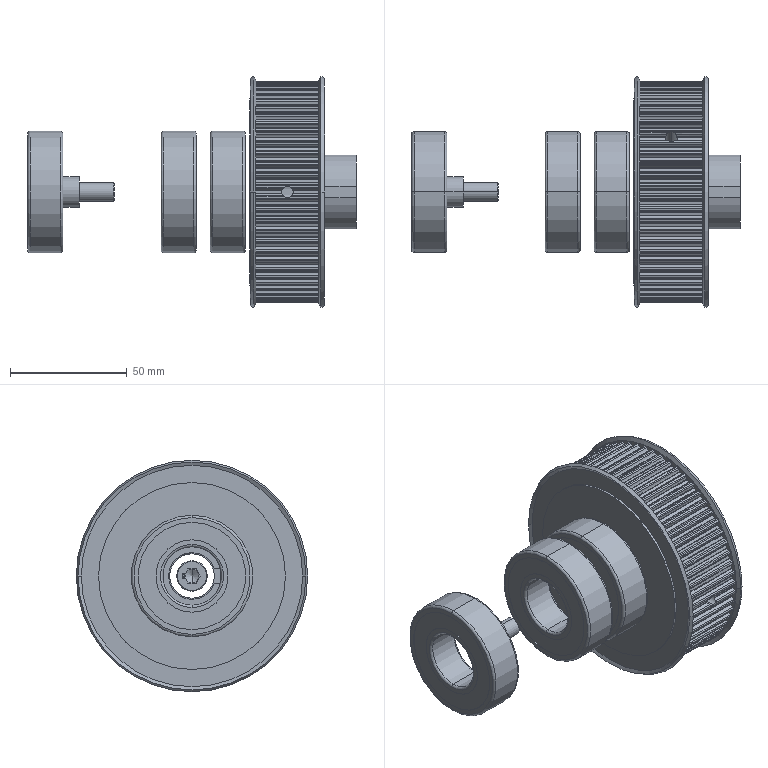Part | NX | 6 solids | 757 faces | box 140.6 x 99 x 99 mm | volume 284136 mm3 | cylinder 582 | plane 133 | torus 24 | cone 18 | commonest cylinder face diameters 0.5 x124 1.1 x124 6.55 x124 94.53 x88 90.99 x63 31 x12